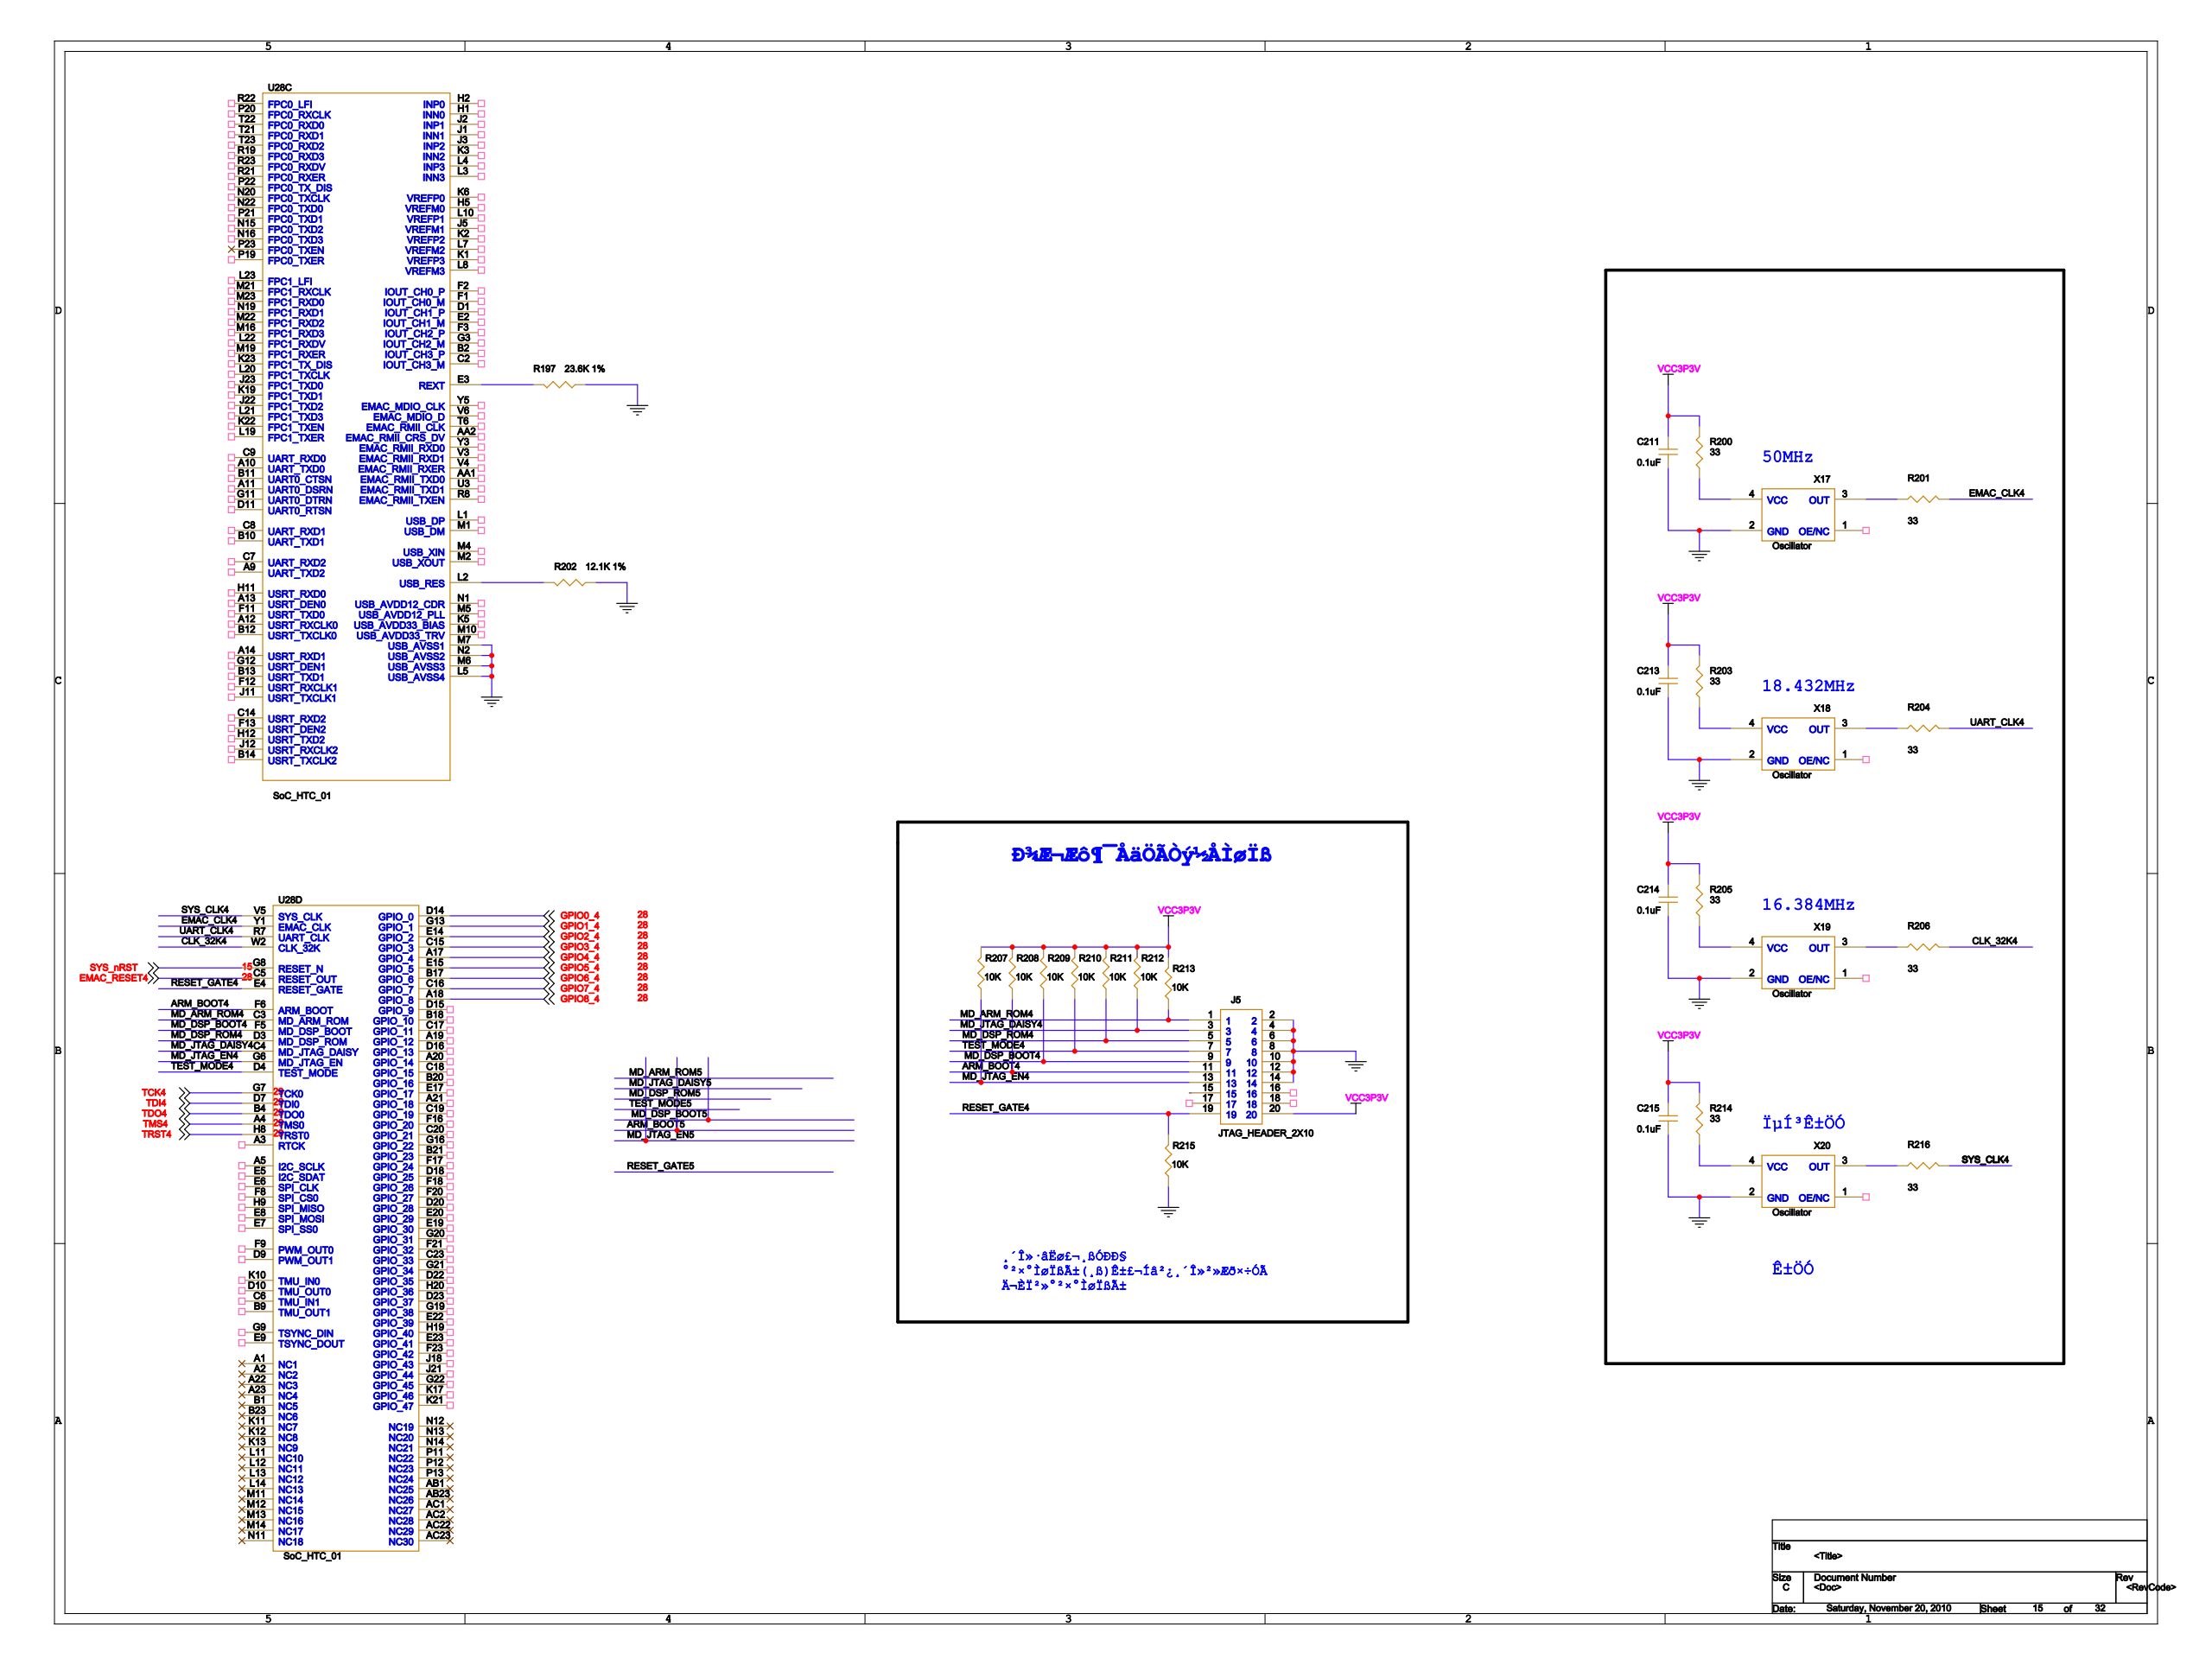Circuit board | Cadence Allegro | 1001 parts | 1318 nets | one sheet of the schematic
Parts on this sheet (reference | value | footprint):
C211 | 0.1uF | 0603
C213 | 0.1uF | 0603
C214 | 0.1uF | 0603
C215 | 0.1uF | 0603
J5 | JTAG_HEADER_2X10 | JTAG_HEADER_2X10
R197 | 23.6K 1% | 0603
R200 | 33 | 0603
R201 | 33 | 0603
R202 | 12.1K 1% | 0603
R203 | 33 | 0603
R204 | 33 | 0603
R205 | 33 | 0603
R206 | 33 | 0603
R207 | 10K | 0603
R208 | 10K | 0603
R209 | 10K | 0603
R210 | 10K | 0603
R211 | 10K | 0603
R212 | 10K | 0603
R213 | 10K | 0603
R214 | 33 | 0603
R215 | 10K | 0603
R216 | 33 | 0603
U28 | SoC_HTC_01 | L529_XIN
X17 | Oscillator | OSC_5_7
X18 | Oscillator | OSC_5_7
X19 | Oscillator | OSC_5_7
X20 | Oscillator | OSC_5_7
Nets of these parts (net: part-pin ...):
GPIO1_4: U28-G13
TCK4: U28-G7
TDO4: U28-B4
EMAC_RESET4: U28-C5
TMS4: U28-A4
TDI4: U28-D7
GPIO5_4: U28-E15
GPIO7_4: U28-C16
GPIO2_4: U28-E14
GPIO6_4: U28-B17
GPIO0_4: U28-D14
GPIO3_4: U28-C15
GPIO4_4: U28-A17
GPIO8_4: U28-A18
TRST4: U28-H8
GND: C211-2 C213-2 C214-2 C215-2 J5-2 J5-4 J5-6 J5-8 J5-10 J5-12 J5-14 R197-1 R202-1 R215-1 X17-2 X18-2 X19-2 X20-2 U28-L5 U28-M6 U28-M7 U28-N2
VCC3P3V: C211-1 C213-1 C214-1 C215-1 J5-20 R200-2 R203-2 R205-2 R207-2 R208-2 R209-2 R210-2 R211-2 R212-2 R213-2 R214-2
N16843025: R197-2 U28-E3
N16843248: R202-2 U28-L2
ARM_BOOT4: J5-11 R208-1 U28-F6
CLK_32K4: R206-2 U28-W2
EMAC_CLK4: R201-2 U28-Y1
MD_ARM_ROM4: J5-1 R213-1 U28-C3
MD_DSP_BOOT4: J5-9 R209-1 U28-F5
MD_DSP_ROM4: J5-5 R211-1 U28-D3
MD_JTAG_DAISY4: J5-3 R212-1 U28-C4
MD_JTAG_EN4: J5-13 R207-1 U28-G6
RESET_GATE4: J5-19 R215-2 U28-E4
SYS_CLK_16842839: R216-2 U28-V5
TEST_MODE4: J5-7 R210-1 U28-D4
UART_CLK4: R204-2 U28-R7
N19060606: J5-15
N16843764: R200-1 X17-4
N16843756: R201-1 X17-3
N16843774: R203-1 X18-4
N16843788: R204-1 X18-3
N16842791: R205-1 X19-4
N16842825: R206-1 X19-3
N16842812: R214-1 X20-4
N16842861: R216-1 X20-3